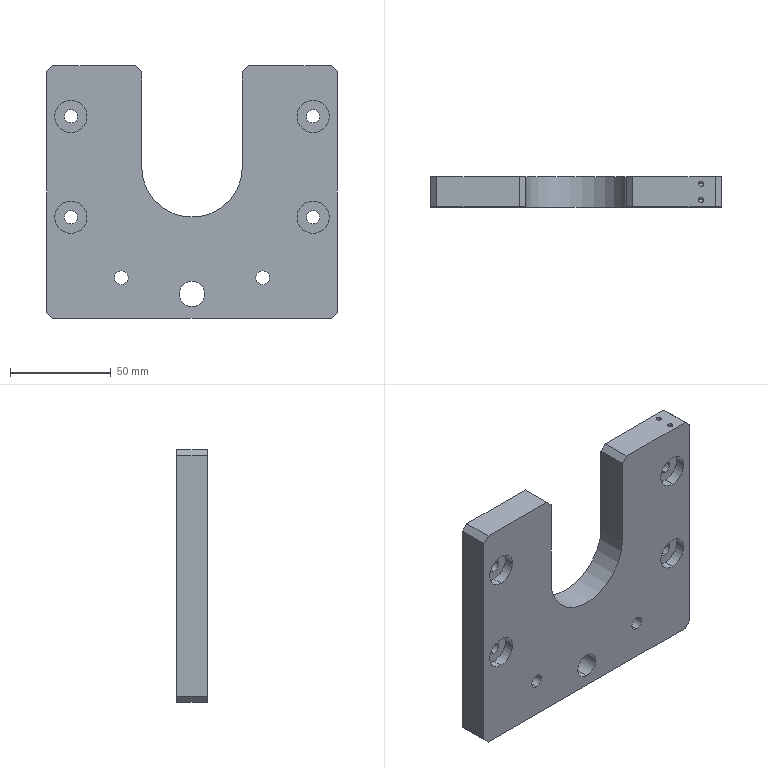Part | STEP file | PN_0003 Plate_Default | 1 solid | 50 faces | box 144 x 15 x 125 mm | volume 209014 mm3 | cylinder 27 | plane 19 | cone 4 | commonest cylinder face diameters 6.5 x8 16 x8 2.5 x4 6.8 x4 12.5 x2 50 x1